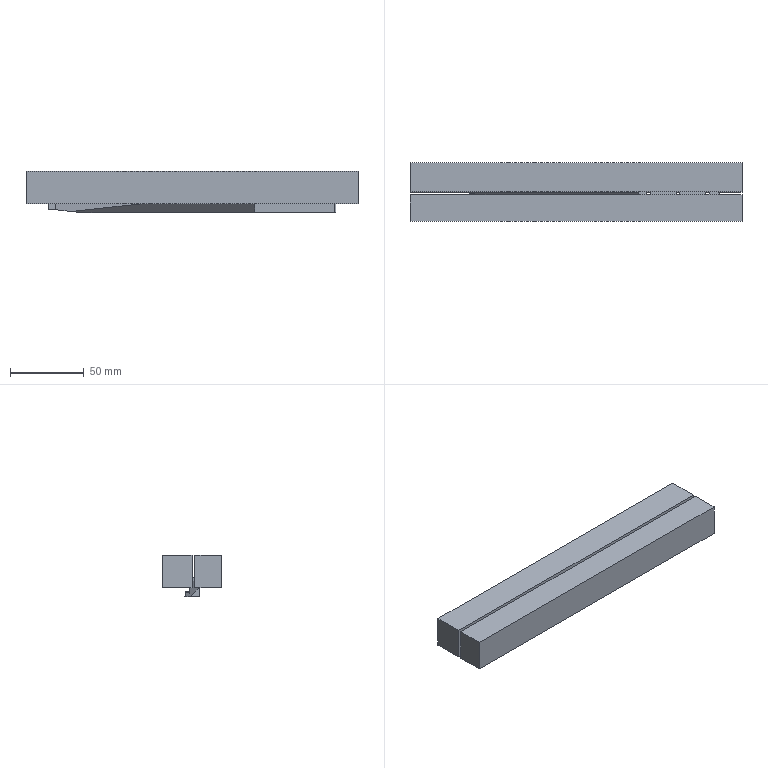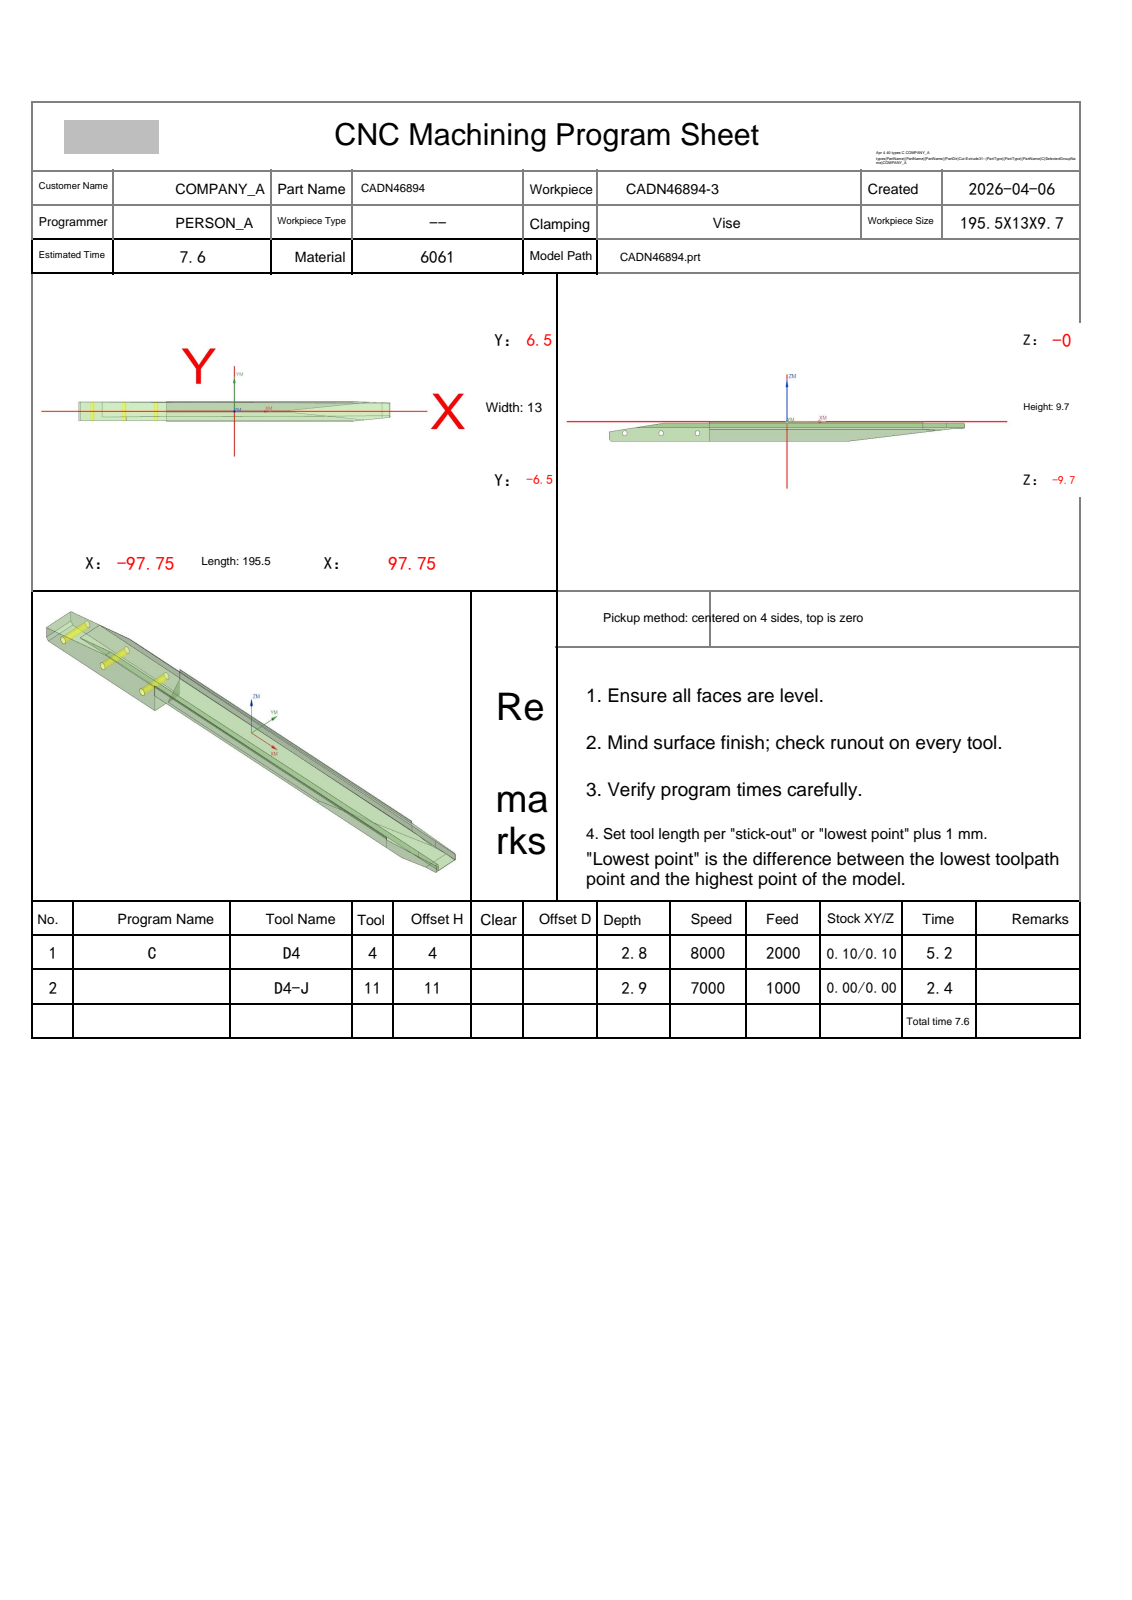NC program | NX | posted by the shop | part box 225.5 x 39.7 x 28 mm
Lines 11943 to 12871 of 20119:
N3 T19 M06
(D1.5-J  D=1.5 R=0. H=19 ce=0.00 di=0.00)
G00 G90 G54 X-194.982 Y-9.122 M03 S8000
G43 H19 Z44.
M08
Z-5.95
G01 X-194.984 Y-9.121 Z-5.973 F800.
X-194.989 Y-9.118 Z-5.993
X-194.996 Y-9.115 Z-6.012
X-195.007 Y-9.11 Z-6.028
X-195.02 Y-9.105 Z-6.042
X-195.034 Y-9.101 Z-6.055
X-195.05 Y-9.097 Z-6.065
X-195.068 Y-9.093 Z-6.074
X-195.086 Y-9.092 Z-6.082
X-195.105 Z-6.088
X-195.124 Y-9.094 Z-6.092
X-195.143 Y-9.099 Z-6.096
X-195.162 Y-9.108 Z-6.098
X-195.179 Y-9.119 Z-6.1
X-195.196 Y-9.135
G02 X-195.625 Y-9.483 I-1.304 J1.167
G03 X-195.75 Y-9.7 I.125 J-.217
X-195.5 Y-9.95 I.25 J0.0
G01 X-195.35 Y-9.9
G02 X-194.869 Y-9.583 I2.85 J-3.8
G01 X-194.848 Y-9.565 Z-6.101
X-194.834 Y-9.541 Z-6.102
X-194.824 Y-9.511 Z-6.105
X-194.82 Y-9.477 Z-6.108
Y-9.442 Z-6.112
X-194.823 Y-9.406 Z-6.117
X-194.828 Y-9.371 Z-6.122
X-194.836 Y-9.338 Z-6.127
X-194.851 Y-9.294 Z-6.136
X-194.871 Y-9.258 Z-6.145
X-194.895 Y-9.227 Z-6.155
X-194.927 Y-9.2 Z-6.164
X-194.966 Y-9.174 Z-6.173
X-194.994 Y-9.157 Z-6.178
X-195.025 Y-9.141 Z-6.183
X-195.057 Y-9.127 Z-6.188
X-195.089 Y-9.117 Z-6.192
X-195.12 Y-9.111 Z-6.195
X-195.149 Z-6.198
X-195.175 Y-9.119 Z-6.199
X-195.196 Y-9.135 Z-6.2
G02 X-195.625 Y-9.483 I-1.304 J1.167
G03 X-195.75 Y-9.7 I.125 J-.217
X-195.5 Y-9.95 I.25 J0.0
G01 X-195.35 Y-9.9
G02 X-194.869 Y-9.583 I2.85 J-3.8
G01 X-194.848 Y-9.565 Z-6.201
X-194.834 Y-9.541 Z-6.202
X-194.824 Y-9.511 Z-6.205
X-194.82 Y-9.477 Z-6.208
Y-9.442 Z-6.212
X-194.823 Y-9.406 Z-6.217
X-194.828 Y-9.371 Z-6.222
X-194.836 Y-9.338 Z-6.227
X-194.851 Y-9.294 Z-6.236
X-194.871 Y-9.258 Z-6.245
X-194.895 Y-9.227 Z-6.255
X-194.927 Y-9.2 Z-6.264
X-194.966 Y-9.174 Z-6.273
X-194.994 Y-9.157 Z-6.278
X-195.025 Y-9.141 Z-6.283
X-195.057 Y-9.127 Z-6.288
X-195.089 Y-9.117 Z-6.292
X-195.12 Y-9.111 Z-6.295
X-195.149 Z-6.298
X-195.175 Y-9.119 Z-6.299
X-195.196 Y-9.135 Z-6.3
G02 X-195.625 Y-9.483 I-1.304 J1.167
G03 X-195.75 Y-9.7 I.125 J-.217
X-195.5 Y-9.95 I.25 J0.0
G01 X-195.35 Y-9.9
G02 X-194.869 Y-9.583 I2.85 J-3.8
G01 X-194.848 Y-9.565 Z-6.301
X-194.834 Y-9.541 Z-6.302
X-194.824 Y-9.511 Z-6.305
X-194.82 Y-9.477 Z-6.308
Y-9.442 Z-6.312
X-194.823 Y-9.406 Z-6.317
X-194.828 Y-9.371 Z-6.322
X-194.836 Y-9.338 Z-6.327
X-194.851 Y-9.294 Z-6.336
X-194.871 Y-9.258 Z-6.345
X-194.895 Y-9.227 Z-6.355
X-194.927 Y-9.2 Z-6.364
X-194.966 Y-9.174 Z-6.373
X-194.994 Y-9.157 Z-6.378
X-195.025 Y-9.141 Z-6.383
X-195.057 Y-9.127 Z-6.388
X-195.089 Y-9.117 Z-6.392
X-195.12 Y-9.111 Z-6.395
X-195.149 Z-6.398
X-195.175 Y-9.119 Z-6.399
X-195.196 Y-9.135 Z-6.4
G02 X-195.625 Y-9.483 I-1.304 J1.167
G03 X-195.75 Y-9.7 I.125 J-.217
X-195.5 Y-9.95 I.25 J0.0
G01 X-195.35 Y-9.9
G02 X-194.869 Y-9.583 I2.85 J-3.8
G01 X-194.848 Y-9.565 Z-6.401
X-194.834 Y-9.541 Z-6.402
X-194.824 Y-9.511 Z-6.405
X-194.82 Y-9.477 Z-6.408
Y-9.442 Z-6.412
X-194.823 Y-9.406 Z-6.417
X-194.828 Y-9.371 Z-6.422
X-194.836 Y-9.338 Z-6.427
X-194.851 Y-9.294 Z-6.436
X-194.871 Y-9.258 Z-6.445
X-194.895 Y-9.227 Z-6.455
X-194.927 Y-9.2 Z-6.464
X-194.966 Y-9.174 Z-6.473
X-194.994 Y-9.157 Z-6.478
X-195.025 Y-9.141 Z-6.483
X-195.057 Y-9.127 Z-6.488
X-195.089 Y-9.117 Z-6.492
X-195.12 Y-9.111 Z-6.495
X-195.149 Z-6.498
X-195.175 Y-9.119 Z-6.499
X-195.196 Y-9.135 Z-6.5
G02 X-195.625 Y-9.483 I-1.304 J1.167
G03 X-195.75 Y-9.7 I.125 J-.217
X-195.5 Y-9.95 I.25 J0.0
G01 X-195.35 Y-9.9
G02 X-194.869 Y-9.583 I2.85 J-3.8
G01 X-194.848 Y-9.565 Z-6.501
X-194.834 Y-9.541 Z-6.502
X-194.824 Y-9.511 Z-6.505
X-194.82 Y-9.477 Z-6.508
Y-9.442 Z-6.512
X-194.823 Y-9.406 Z-6.517
X-194.828 Y-9.371 Z-6.522
X-194.836 Y-9.338 Z-6.527
X-194.851 Y-9.294 Z-6.536
X-194.871 Y-9.258 Z-6.545
X-194.895 Y-9.227 Z-6.555
X-194.927 Y-9.2 Z-6.564
X-194.966 Y-9.174 Z-6.573
X-194.994 Y-9.157 Z-6.578
X-195.025 Y-9.141 Z-6.583
X-195.057 Y-9.127 Z-6.588
X-195.089 Y-9.117 Z-6.592
X-195.12 Y-9.111 Z-6.595
X-195.149 Z-6.598
X-195.175 Y-9.119 Z-6.599
X-195.196 Y-9.135 Z-6.6
G02 X-195.625 Y-9.483 I-1.304 J1.167
G03 X-195.75 Y-9.7 I.125 J-.217
X-195.5 Y-9.95 I.25 J0.0
G01 X-195.35 Y-9.9
G02 X-194.869 Y-9.583 I2.85 J-3.8
G01 X-194.848 Y-9.565 Z-6.601
X-194.834 Y-9.541 Z-6.602
X-194.824 Y-9.511 Z-6.605
X-194.82 Y-9.477 Z-6.608
Y-9.442 Z-6.612
X-194.823 Y-9.406 Z-6.617
X-194.828 Y-9.371 Z-6.622
X-194.836 Y-9.338 Z-6.627
X-194.851 Y-9.294 Z-6.636
X-194.871 Y-9.258 Z-6.645
X-194.895 Y-9.227 Z-6.655
X-194.927 Y-9.2 Z-6.664
X-194.966 Y-9.174 Z-6.673
X-194.994 Y-9.157 Z-6.678
X-195.025 Y-9.141 Z-6.683
X-195.057 Y-9.127 Z-6.688
X-195.089 Y-9.117 Z-6.692
X-195.12 Y-9.111 Z-6.695
X-195.149 Z-6.698
X-195.175 Y-9.119 Z-6.699
X-195.196 Y-9.135 Z-6.7
G02 X-195.625 Y-9.483 I-1.304 J1.167
G03 X-195.75 Y-9.7 I.125 J-.217
X-195.5 Y-9.95 I.25 J0.0
G01 X-195.35 Y-9.9
G02 X-194.869 Y-9.583 I2.85 J-3.8
G01 X-194.848 Y-9.565 Z-6.701
X-194.834 Y-9.541 Z-6.702
X-194.824 Y-9.511 Z-6.705
X-194.82 Y-9.477 Z-6.708
Y-9.442 Z-6.712
X-194.823 Y-9.406 Z-6.717
X-194.828 Y-9.371 Z-6.722
X-194.836 Y-9.338 Z-6.727
X-194.851 Y-9.294 Z-6.736
X-194.871 Y-9.258 Z-6.745
X-194.895 Y-9.227 Z-6.755
X-194.927 Y-9.2 Z-6.764
X-194.966 Y-9.174 Z-6.773
X-194.994 Y-9.157 Z-6.778
X-195.025 Y-9.141 Z-6.783
X-195.057 Y-9.127 Z-6.788
X-195.089 Y-9.117 Z-6.792
X-195.12 Y-9.111 Z-6.795
X-195.149 Z-6.798
X-195.175 Y-9.119 Z-6.799
X-195.196 Y-9.135 Z-6.8
G02 X-195.625 Y-9.483 I-1.304 J1.167
G03 X-195.75 Y-9.7 I.125 J-.217
X-195.5 Y-9.95 I.25 J0.0
G01 X-195.35 Y-9.9
G02 X-194.869 Y-9.583 I2.85 J-3.8
G01 X-194.848 Y-9.565 Z-6.801
X-194.834 Y-9.541 Z-6.802
X-194.824 Y-9.511 Z-6.805
X-194.82 Y-9.477 Z-6.808
Y-9.442 Z-6.812
X-194.823 Y-9.406 Z-6.817
X-194.828 Y-9.371 Z-6.822
X-194.836 Y-9.338 Z-6.827
X-194.851 Y-9.294 Z-6.836
X-194.871 Y-9.258 Z-6.845
X-194.895 Y-9.227 Z-6.855
X-194.927 Y-9.2 Z-6.864
X-194.966 Y-9.174 Z-6.873
X-194.994 Y-9.157 Z-6.878
X-195.025 Y-9.141 Z-6.883
X-195.057 Y-9.127 Z-6.888
X-195.089 Y-9.117 Z-6.892
X-195.12 Y-9.111 Z-6.895
X-195.149 Z-6.898
X-195.175 Y-9.119 Z-6.899
X-195.196 Y-9.135 Z-6.9
G02 X-195.625 Y-9.483 I-1.304 J1.167
G03 X-195.75 Y-9.7 I.125 J-.217
X-195.5 Y-9.95 I.25 J0.0
G01 X-195.35 Y-9.9
G02 X-194.869 Y-9.583 I2.85 J-3.8
G01 X-194.848 Y-9.565 Z-6.901
X-194.834 Y-9.541 Z-6.902
X-194.824 Y-9.511 Z-6.905
X-194.82 Y-9.477 Z-6.908
Y-9.442 Z-6.912
X-194.823 Y-9.406 Z-6.917
X-194.828 Y-9.371 Z-6.922
X-194.836 Y-9.338 Z-6.927
X-194.851 Y-9.294 Z-6.936
X-194.871 Y-9.258 Z-6.945
X-194.895 Y-9.227 Z-6.955
X-194.927 Y-9.2 Z-6.964
X-194.966 Y-9.174 Z-6.973
X-194.994 Y-9.157 Z-6.978
X-195.025 Y-9.141 Z-6.983
X-195.057 Y-9.127 Z-6.988
X-195.089 Y-9.117 Z-6.992
X-195.12 Y-9.111 Z-6.995
X-195.149 Z-6.998
X-195.175 Y-9.119 Z-6.999
X-195.196 Y-9.135 Z-7.
G02 X-195.625 Y-9.483 I-1.304 J1.167
G03 X-195.75 Y-9.7 I.125 J-.217
X-195.5 Y-9.95 I.25 J0.0
G01 X-195.35 Y-9.9
G02 X-194.869 Y-9.583 I2.85 J-3.8
G01 X-194.848 Y-9.565 Z-7.001
X-194.834 Y-9.541 Z-7.002
X-194.824 Y-9.511 Z-7.005
X-194.82 Y-9.477 Z-7.008
Y-9.442 Z-7.012
X-194.823 Y-9.406 Z-7.017
X-194.828 Y-9.371 Z-7.022
X-194.836 Y-9.338 Z-7.027
X-194.851 Y-9.294 Z-7.036
X-194.871 Y-9.258 Z-7.045
X-194.895 Y-9.227 Z-7.055
X-194.927 Y-9.2 Z-7.064
X-194.966 Y-9.174 Z-7.073
X-194.994 Y-9.157 Z-7.078
X-195.025 Y-9.141 Z-7.083
X-195.057 Y-9.127 Z-7.088
X-195.089 Y-9.117 Z-7.092
X-195.12 Y-9.111 Z-7.095
X-195.149 Z-7.098
X-195.175 Y-9.119 Z-7.099
X-195.196 Y-9.135 Z-7.1
G02 X-195.625 Y-9.483 I-1.304 J1.167
G03 X-195.75 Y-9.7 I.125 J-.217
X-195.5 Y-9.95 I.25 J0.0
G01 X-195.35 Y-9.9
G02 X-194.869 Y-9.583 I2.85 J-3.8
G01 X-194.848 Y-9.565 Z-7.101
X-194.834 Y-9.541 Z-7.102
X-194.824 Y-9.511 Z-7.105
X-194.82 Y-9.477 Z-7.108
Y-9.442 Z-7.112
X-194.823 Y-9.406 Z-7.117
X-194.828 Y-9.371 Z-7.122
X-194.836 Y-9.338 Z-7.127
X-194.851 Y-9.294 Z-7.136
X-194.871 Y-9.258 Z-7.145
X-194.895 Y-9.227 Z-7.155
X-194.927 Y-9.2 Z-7.164
X-194.966 Y-9.174 Z-7.173
X-194.994 Y-9.157 Z-7.178
X-195.025 Y-9.141 Z-7.183
X-195.057 Y-9.127 Z-7.188
X-195.089 Y-9.117 Z-7.192
X-195.12 Y-9.111 Z-7.195
X-195.149 Z-7.198
X-195.175 Y-9.119 Z-7.199
X-195.196 Y-9.135 Z-7.2
G02 X-195.625 Y-9.483 I-1.304 J1.167
G03 X-195.75 Y-9.7 I.125 J-.217
X-195.5 Y-9.95 I.25 J0.0
G01 X-195.35 Y-9.9
G02 X-194.869 Y-9.583 I2.85 J-3.8
G01 X-194.848 Y-9.565 Z-7.201
X-194.834 Y-9.541 Z-7.202
X-194.824 Y-9.511 Z-7.205
X-194.82 Y-9.477 Z-7.208
Y-9.442 Z-7.212
X-194.823 Y-9.406 Z-7.217
X-194.828 Y-9.371 Z-7.222
X-194.836 Y-9.338 Z-7.227
X-194.851 Y-9.294 Z-7.236
X-194.871 Y-9.258 Z-7.245
X-194.895 Y-9.227 Z-7.255
X-194.927 Y-9.2 Z-7.264
X-194.966 Y-9.174 Z-7.273
X-194.994 Y-9.157 Z-7.278
X-195.025 Y-9.141 Z-7.283
X-195.057 Y-9.127 Z-7.288
X-195.089 Y-9.117 Z-7.292
X-195.12 Y-9.111 Z-7.295
X-195.149 Z-7.298
X-195.175 Y-9.119 Z-7.299
X-195.196 Y-9.135 Z-7.3
G02 X-195.625 Y-9.483 I-1.304 J1.167
G03 X-195.75 Y-9.7 I.125 J-.217
X-195.5 Y-9.95 I.25 J0.0
G01 X-195.35 Y-9.9
G02 X-194.869 Y-9.583 I2.85 J-3.8
G01 X-194.848 Y-9.565 Z-7.301
X-194.834 Y-9.541 Z-7.302
X-194.824 Y-9.511 Z-7.305
X-194.82 Y-9.477 Z-7.308
Y-9.442 Z-7.312
X-194.823 Y-9.406 Z-7.317
X-194.828 Y-9.371 Z-7.322
X-194.836 Y-9.338 Z-7.327
X-194.851 Y-9.294 Z-7.336
X-194.871 Y-9.258 Z-7.345
X-194.895 Y-9.227 Z-7.355
X-194.927 Y-9.2 Z-7.364
X-194.966 Y-9.174 Z-7.373
X-194.994 Y-9.157 Z-7.378
X-195.025 Y-9.141 Z-7.383
X-195.057 Y-9.127 Z-7.388
X-195.089 Y-9.117 Z-7.392
X-195.12 Y-9.111 Z-7.395
X-195.149 Z-7.398
X-195.175 Y-9.119 Z-7.399
X-195.196 Y-9.135 Z-7.4
G02 X-195.625 Y-9.483 I-1.304 J1.167
G03 X-195.75 Y-9.7 I.125 J-.217
X-195.5 Y-9.95 I.25 J0.0
G01 X-195.35 Y-9.9
G02 X-194.869 Y-9.583 I2.85 J-3.8
G01 X-194.848 Y-9.565 Z-7.401
X-194.834 Y-9.541 Z-7.402
X-194.824 Y-9.511 Z-7.405
X-194.82 Y-9.477 Z-7.408
Y-9.442 Z-7.412
X-194.823 Y-9.406 Z-7.417
X-194.828 Y-9.371 Z-7.422
X-194.836 Y-9.338 Z-7.427
X-194.851 Y-9.294 Z-7.436
X-194.871 Y-9.258 Z-7.445
X-194.895 Y-9.227 Z-7.455
X-194.927 Y-9.2 Z-7.464
X-194.966 Y-9.174 Z-7.473
X-194.994 Y-9.157 Z-7.478
X-195.025 Y-9.141 Z-7.483
X-195.057 Y-9.127 Z-7.488
X-195.089 Y-9.117 Z-7.492
X-195.12 Y-9.111 Z-7.495
X-195.149 Z-7.498
X-195.175 Y-9.119 Z-7.499
X-195.196 Y-9.135 Z-7.5
G02 X-195.625 Y-9.483 I-1.304 J1.167
G03 X-195.75 Y-9.7 I.125 J-.217
X-195.5 Y-9.95 I.25 J0.0
G01 X-195.35 Y-9.9
G02 X-194.869 Y-9.583 I2.85 J-3.8
G01 X-194.848 Y-9.565 Z-7.501
X-194.834 Y-9.541 Z-7.502
X-194.824 Y-9.511 Z-7.505
X-194.82 Y-9.477 Z-7.508
Y-9.442 Z-7.512
X-194.823 Y-9.406 Z-7.517
X-194.828 Y-9.371 Z-7.522
X-194.836 Y-9.338 Z-7.527
X-194.851 Y-9.294 Z-7.536
X-194.871 Y-9.258 Z-7.545
X-194.895 Y-9.227 Z-7.555
X-194.927 Y-9.2 Z-7.564
X-194.966 Y-9.174 Z-7.573
X-194.994 Y-9.157 Z-7.578
X-195.025 Y-9.141 Z-7.583
X-195.057 Y-9.127 Z-7.588
X-195.089 Y-9.117 Z-7.592
X-195.12 Y-9.111 Z-7.595
X-195.149 Z-7.598
X-195.175 Y-9.119 Z-7.599
X-195.196 Y-9.135 Z-7.6
G02 X-195.625 Y-9.483 I-1.304 J1.167
G03 X-195.75 Y-9.7 I.125 J-.217
X-195.5 Y-9.95 I.25 J0.0
G01 X-195.35 Y-9.9
G02 X-194.869 Y-9.583 I2.85 J-3.8
G01 X-194.848 Y-9.565 Z-7.601
X-194.834 Y-9.541 Z-7.602
X-194.824 Y-9.511 Z-7.605
X-194.82 Y-9.477 Z-7.608
Y-9.442 Z-7.612
X-194.823 Y-9.406 Z-7.617
X-194.828 Y-9.371 Z-7.622
X-194.836 Y-9.338 Z-7.627
X-194.851 Y-9.294 Z-7.636
X-194.871 Y-9.258 Z-7.645
X-194.895 Y-9.227 Z-7.655
X-194.927 Y-9.2 Z-7.664
X-194.966 Y-9.174 Z-7.673
X-194.994 Y-9.157 Z-7.678
X-195.025 Y-9.141 Z-7.683
X-195.057 Y-9.127 Z-7.688
X-195.089 Y-9.117 Z-7.692
X-195.12 Y-9.111 Z-7.695
X-195.149 Z-7.698
X-195.175 Y-9.119 Z-7.699
X-195.196 Y-9.135 Z-7.7
G02 X-195.625 Y-9.483 I-1.304 J1.167
G03 X-195.75 Y-9.7 I.125 J-.217
X-195.5 Y-9.95 I.25 J0.0
G01 X-195.35 Y-9.9
G02 X-194.869 Y-9.583 I2.85 J-3.8
G01 X-194.848 Y-9.565 Z-7.701
X-194.834 Y-9.541 Z-7.702
X-194.824 Y-9.511 Z-7.705
X-194.82 Y-9.477 Z-7.708
Y-9.442 Z-7.712
X-194.823 Y-9.406 Z-7.717
X-194.828 Y-9.371 Z-7.722
X-194.836 Y-9.338 Z-7.727
X-194.851 Y-9.294 Z-7.736
X-194.871 Y-9.258 Z-7.745
X-194.895 Y-9.227 Z-7.755
X-194.927 Y-9.2 Z-7.764
X-194.966 Y-9.174 Z-7.773
X-194.994 Y-9.157 Z-7.778
X-195.025 Y-9.141 Z-7.783
X-195.057 Y-9.127 Z-7.788
X-195.089 Y-9.117 Z-7.792
X-195.12 Y-9.111 Z-7.795
X-195.149 Z-7.798
X-195.175 Y-9.119 Z-7.799
X-195.196 Y-9.135 Z-7.8
G02 X-195.625 Y-9.483 I-1.304 J1.167
G03 X-195.75 Y-9.7 I.125 J-.217
X-195.5 Y-9.95 I.25 J0.0
G01 X-195.35 Y-9.9
G02 X-194.869 Y-9.583 I2.85 J-3.8
G01 X-194.848 Y-9.565 Z-7.801
X-194.834 Y-9.541 Z-7.802
X-194.824 Y-9.511 Z-7.805
X-194.82 Y-9.477 Z-7.808
Y-9.442 Z-7.812
X-194.823 Y-9.406 Z-7.817
X-194.828 Y-9.371 Z-7.822
X-194.836 Y-9.338 Z-7.827
X-194.851 Y-9.294 Z-7.836
X-194.871 Y-9.258 Z-7.845
X-194.895 Y-9.227 Z-7.855
X-194.927 Y-9.2 Z-7.864
X-194.966 Y-9.174 Z-7.873
X-194.994 Y-9.157 Z-7.878
X-195.025 Y-9.141 Z-7.883
X-195.057 Y-9.127 Z-7.888
X-195.089 Y-9.117 Z-7.892
X-195.12 Y-9.111 Z-7.895
X-195.149 Z-7.898
X-195.175 Y-9.119 Z-7.899
X-195.196 Y-9.135 Z-7.9
G02 X-195.625 Y-9.483 I-1.304 J1.167
G03 X-195.75 Y-9.7 I.125 J-.217
X-195.5 Y-9.95 I.25 J0.0
G01 X-195.35 Y-9.9
G02 X-194.869 Y-9.583 I2.85 J-3.8
G01 X-194.848 Y-9.565 Z-7.901
X-194.834 Y-9.541 Z-7.902
X-194.824 Y-9.511 Z-7.905
X-194.82 Y-9.477 Z-7.908
Y-9.442 Z-7.912
X-194.823 Y-9.406 Z-7.917
X-194.828 Y-9.371 Z-7.922
X-194.836 Y-9.338 Z-7.927
X-194.851 Y-9.294 Z-7.936
X-194.871 Y-9.258 Z-7.945
X-194.895 Y-9.227 Z-7.955
X-194.927 Y-9.2 Z-7.964
X-194.966 Y-9.174 Z-7.973
X-194.994 Y-9.157 Z-7.978
X-195.025 Y-9.141 Z-7.983
X-195.057 Y-9.127 Z-7.988
X-195.089 Y-9.117 Z-7.992
X-195.12 Y-9.111 Z-7.995
X-195.149 Z-7.998
X-195.175 Y-9.119 Z-7.999
X-195.196 Y-9.135 Z-8.
G02 X-195.625 Y-9.483 I-1.304 J1.167
G03 X-195.75 Y-9.7 I.125 J-.217
X-195.5 Y-9.95 I.25 J0.0
G01 X-195.35 Y-9.9
G02 X-194.869 Y-9.583 I2.85 J-3.8
G01 X-194.848 Y-9.565 Z-8.001
X-194.834 Y-9.541 Z-8.002
X-194.824 Y-9.511 Z-8.005
X-194.82 Y-9.477 Z-8.008
Y-9.442 Z-8.012
X-194.823 Y-9.406 Z-8.017
X-194.828 Y-9.371 Z-8.022
X-194.836 Y-9.338 Z-8.027
X-194.851 Y-9.294 Z-8.036
X-194.871 Y-9.258 Z-8.045
X-194.895 Y-9.227 Z-8.055
X-194.927 Y-9.2 Z-8.064
X-194.966 Y-9.174 Z-8.073
X-194.994 Y-9.157 Z-8.078
X-195.025 Y-9.141 Z-8.083
X-195.057 Y-9.127 Z-8.088
X-195.089 Y-9.117 Z-8.092
X-195.12 Y-9.111 Z-8.095
X-195.149 Z-8.098
X-195.175 Y-9.119 Z-8.099
X-195.196 Y-9.135 Z-8.1
G02 X-195.625 Y-9.483 I-1.304 J1.167
G03 X-195.75 Y-9.7 I.125 J-.217
X-195.5 Y-9.95 I.25 J0.0
G01 X-195.35 Y-9.9
G02 X-194.869 Y-9.583 I2.85 J-3.8
G01 X-194.848 Y-9.565 Z-8.101
X-194.834 Y-9.541 Z-8.102
X-194.824 Y-9.511 Z-8.105
X-194.82 Y-9.477 Z-8.108
Y-9.442 Z-8.112
X-194.823 Y-9.406 Z-8.117
X-194.828 Y-9.371 Z-8.122
X-194.836 Y-9.338 Z-8.127
X-194.851 Y-9.294 Z-8.136
X-194.871 Y-9.258 Z-8.145
X-194.895 Y-9.227 Z-8.155
X-194.927 Y-9.2 Z-8.164
X-194.966 Y-9.174 Z-8.173
X-194.994 Y-9.157 Z-8.178
X-195.025 Y-9.141 Z-8.183
X-195.057 Y-9.127 Z-8.188
X-195.089 Y-9.117 Z-8.192
X-195.12 Y-9.111 Z-8.195
X-195.149 Z-8.198
X-195.175 Y-9.119 Z-8.199
X-195.196 Y-9.135 Z-8.2
G02 X-195.625 Y-9.483 I-1.304 J1.167
G03 X-195.75 Y-9.7 I.125 J-.217
X-195.5 Y-9.95 I.25 J0.0
G01 X-195.35 Y-9.9
G02 X-194.869 Y-9.583 I2.85 J-3.8
G01 X-194.848 Y-9.565 Z-8.201
X-194.834 Y-9.541 Z-8.202
X-194.824 Y-9.511 Z-8.205
X-194.82 Y-9.477 Z-8.208
Y-9.442 Z-8.212
X-194.823 Y-9.406 Z-8.217
X-194.828 Y-9.371 Z-8.222
X-194.836 Y-9.338 Z-8.227
X-194.851 Y-9.294 Z-8.236
X-194.871 Y-9.258 Z-8.245
X-194.895 Y-9.227 Z-8.255
X-194.927 Y-9.2 Z-8.264
X-194.966 Y-9.174 Z-8.273
X-194.994 Y-9.157 Z-8.278
X-195.025 Y-9.141 Z-8.283
X-195.057 Y-9.127 Z-8.288
X-195.089 Y-9.117 Z-8.292
X-195.12 Y-9.111 Z-8.295
X-195.149 Z-8.298
X-195.175 Y-9.119 Z-8.299
X-195.196 Y-9.135 Z-8.3
G02 X-195.625 Y-9.483 I-1.304 J1.167
G03 X-195.75 Y-9.7 I.125 J-.217
X-195.5 Y-9.95 I.25 J0.0
G01 X-195.35 Y-9.9
G02 X-194.869 Y-9.583 I2.85 J-3.8
G01 X-194.848 Y-9.565 Z-8.301
X-194.834 Y-9.541 Z-8.302
X-194.824 Y-9.511 Z-8.305
X-194.82 Y-9.477 Z-8.308
Y-9.442 Z-8.312
X-194.823 Y-9.406 Z-8.317
X-194.828 Y-9.371 Z-8.322
X-194.836 Y-9.338 Z-8.327
X-194.851 Y-9.294 Z-8.336
X-194.871 Y-9.258 Z-8.345
X-194.895 Y-9.227 Z-8.355
X-194.927 Y-9.2 Z-8.364
X-194.966 Y-9.174 Z-8.373
X-194.994 Y-9.157 Z-8.378
X-195.025 Y-9.141 Z-8.383
X-195.057 Y-9.127 Z-8.388
X-195.089 Y-9.117 Z-8.392
X-195.12 Y-9.111 Z-8.395
X-195.149 Z-8.398
X-195.175 Y-9.119 Z-8.399
X-195.196 Y-9.135 Z-8.4
G02 X-195.625 Y-9.483 I-1.304 J1.167
G03 X-195.75 Y-9.7 I.125 J-.217
X-195.5 Y-9.95 I.25 J0.0
G01 X-195.35 Y-9.9
G02 X-194.869 Y-9.583 I2.85 J-3.8
G01 X-194.848 Y-9.565 Z-8.401
X-194.834 Y-9.541 Z-8.402
X-194.824 Y-9.511 Z-8.405
X-194.82 Y-9.477 Z-8.408
Y-9.442 Z-8.412
X-194.823 Y-9.406 Z-8.417
X-194.828 Y-9.371 Z-8.422
X-194.836 Y-9.338 Z-8.427
X-194.851 Y-9.294 Z-8.436
X-194.871 Y-9.258 Z-8.445
X-194.895 Y-9.227 Z-8.455
X-194.927 Y-9.2 Z-8.464
X-194.966 Y-9.174 Z-8.473
X-194.994 Y-9.157 Z-8.478
X-195.025 Y-9.141 Z-8.483
X-195.057 Y-9.127 Z-8.488
X-195.089 Y-9.117 Z-8.492
X-195.12 Y-9.111 Z-8.495
X-195.149 Z-8.498
X-195.175 Y-9.119 Z-8.499
X-195.196 Y-9.135 Z-8.5
G02 X-195.625 Y-9.483 I-1.304 J1.167
G03 X-195.75 Y-9.7 I.125 J-.217
X-195.5 Y-9.95 I.25 J0.0
G01 X-195.35 Y-9.9
G02 X-194.869 Y-9.583 I2.85 J-3.8
G01 X-194.848 Y-9.565 Z-8.501
X-194.834 Y-9.541 Z-8.502
X-194.824 Y-9.511 Z-8.505
X-194.82 Y-9.477 Z-8.508
Y-9.442 Z-8.512
X-194.823 Y-9.406 Z-8.517
X-194.828 Y-9.371 Z-8.522
X-194.836 Y-9.338 Z-8.527
X-194.851 Y-9.294 Z-8.536
X-194.871 Y-9.258 Z-8.545
X-194.895 Y-9.227 Z-8.555
X-194.927 Y-9.2 Z-8.564
X-194.966 Y-9.174 Z-8.573
X-194.994 Y-9.157 Z-8.578
X-195.025 Y-9.141 Z-8.583
X-195.057 Y-9.127 Z-8.588
X-195.089 Y-9.117 Z-8.592
X-195.12 Y-9.111 Z-8.595
X-195.149 Z-8.598
X-195.175 Y-9.119 Z-8.599
X-195.196 Y-9.135 Z-8.6
G02 X-195.625 Y-9.483 I-1.304 J1.167
G03 X-195.75 Y-9.7 I.125 J-.217
X-195.5 Y-9.95 I.25 J0.0
G01 X-195.35 Y-9.9
G02 X-194.869 Y-9.583 I2.85 J-3.8
G01 X-194.848 Y-9.565 Z-8.601
X-194.834 Y-9.541 Z-8.602
X-194.824 Y-9.511 Z-8.605
X-194.82 Y-9.477 Z-8.608
Y-9.442 Z-8.612
X-194.823 Y-9.406 Z-8.617
X-194.828 Y-9.371 Z-8.622
X-194.836 Y-9.338 Z-8.627
X-194.851 Y-9.294 Z-8.636
X-194.871 Y-9.258 Z-8.645
X-194.895 Y-9.227 Z-8.655
X-194.927 Y-9.2 Z-8.664
X-194.966 Y-9.174 Z-8.673
X-194.994 Y-9.157 Z-8.678
X-195.025 Y-9.141 Z-8.683
X-195.057 Y-9.127 Z-8.688
X-195.089 Y-9.117 Z-8.692
X-195.12 Y-9.111 Z-8.695
X-195.149 Z-8.698
X-195.175 Y-9.119 Z-8.699
X-195.196 Y-9.135 Z-8.7
G02 X-195.625 Y-9.483 I-1.304 J1.167
G03 X-195.75 Y-9.7 I.125 J-.217
X-195.5 Y-9.95 I.25 J0.0
G01 X-195.35 Y-9.9
G02 X-194.869 Y-9.583 I2.85 J-3.8
G01 X-194.848 Y-9.565 Z-8.701
X-194.834 Y-9.541 Z-8.702
X-194.824 Y-9.511 Z-8.705
X-194.82 Y-9.477 Z-8.708
Y-9.442 Z-8.712
X-194.823 Y-9.406 Z-8.717
X-194.828 Y-9.371 Z-8.722
X-194.836 Y-9.338 Z-8.727
X-194.851 Y-9.294 Z-8.736
X-194.871 Y-9.258 Z-8.745
X-194.895 Y-9.227 Z-8.755
X-194.927 Y-9.2 Z-8.764
X-194.966 Y-9.174 Z-8.773
X-194.994 Y-9.157 Z-8.778
X-195.025 Y-9.141 Z-8.783
X-195.057 Y-9.127 Z-8.788
X-195.089 Y-9.117 Z-8.792
X-195.12 Y-9.111 Z-8.795
X-195.149 Z-8.798
X-195.175 Y-9.119 Z-8.799
X-195.196 Y-9.135 Z-8.8
G02 X-195.625 Y-9.483 I-1.304 J1.167
G03 X-195.75 Y-9.7 I.125 J-.217
X-195.5 Y-9.95 I.25 J0.0
G01 X-195.35 Y-9.9
G02 X-194.869 Y-9.583 I2.85 J-3.8
G01 X-194.848 Y-9.565 Z-8.801
X-194.834 Y-9.541 Z-8.802
X-194.824 Y-9.511 Z-8.805
X-194.82 Y-9.477 Z-8.808
Y-9.442 Z-8.812
X-194.823 Y-9.406 Z-8.817
X-194.828 Y-9.371 Z-8.822
X-194.836 Y-9.338 Z-8.827
X-194.851 Y-9.294 Z-8.836
X-194.871 Y-9.258 Z-8.845
X-194.895 Y-9.227 Z-8.855
X-194.927 Y-9.2 Z-8.864
X-194.966 Y-9.174 Z-8.873
X-194.994 Y-9.157 Z-8.878
X-195.025 Y-9.141 Z-8.883
X-195.057 Y-9.127 Z-8.888
X-195.089 Y-9.117 Z-8.892
X-195.12 Y-9.111 Z-8.895
X-195.149 Z-8.898
X-195.175 Y-9.119 Z-8.899
X-195.196 Y-9.135 Z-8.9
G02 X-195.625 Y-9.483 I-1.304 J1.167
G03 X-195.75 Y-9.7 I.125 J-.217
X-195.5 Y-9.95 I.25 J0.0
G01 X-195.35 Y-9.9
G02 X-194.869 Y-9.583 I2.85 J-3.8
G01 X-194.848 Y-9.565 Z-8.901
X-194.834 Y-9.541 Z-8.902
X-194.824 Y-9.511 Z-8.905
X-194.82 Y-9.477 Z-8.908
Y-9.442 Z-8.912
X-194.823 Y-9.406 Z-8.917
X-194.828 Y-9.371 Z-8.922
X-194.836 Y-9.338 Z-8.927
X-194.851 Y-9.294 Z-8.936
X-194.871 Y-9.258 Z-8.945
X-194.895 Y-9.227 Z-8.955
X-194.927 Y-9.2 Z-8.964
X-194.966 Y-9.174 Z-8.973
X-194.994 Y-9.157 Z-8.978
X-195.025 Y-9.141 Z-8.983
X-195.057 Y-9.127 Z-8.988
X-195.089 Y-9.117 Z-8.992
X-195.12 Y-9.111 Z-8.995
X-195.149 Z-8.998
X-195.175 Y-9.119 Z-8.999
X-195.196 Y-9.135 Z-9.
G02 X-195.625 Y-9.483 I-1.304 J1.167
G03 X-195.75 Y-9.7 I.125 J-.217
X-195.5 Y-9.95 I.25 J0.0
G01 X-195.35 Y-9.9
G02 X-194.869 Y-9.583 I2.85 J-3.8
G01 X-194.848 Y-9.565 Z-9.001
X-194.834 Y-9.541 Z-9.002
X-194.824 Y-9.511 Z-9.005
X-194.82 Y-9.477 Z-9.008
Y-9.442 Z-9.012
X-194.823 Y-9.406 Z-9.017
X-194.828 Y-9.371 Z-9.022
X-194.836 Y-9.338 Z-9.027
X-194.851 Y-9.294 Z-9.036
X-194.871 Y-9.258 Z-9.045
X-194.895 Y-9.227 Z-9.055
X-194.927 Y-9.2 Z-9.064
X-194.966 Y-9.174 Z-9.073
X-194.994 Y-9.157 Z-9.078
X-195.025 Y-9.141 Z-9.083
X-195.057 Y-9.127 Z-9.088
X-195.089 Y-9.117 Z-9.092
X-195.12 Y-9.111 Z-9.095
X-195.149 Z-9.098
X-195.175 Y-9.119 Z-9.099
X-195.196 Y-9.135 Z-9.1
G02 X-195.625 Y-9.483 I-1.304 J1.167
G03 X-195.75 Y-9.7 I.125 J-.217
X-195.5 Y-9.95 I.25 J0.0
G01 X-195.35 Y-9.9
G02 X-194.869 Y-9.583 I2.85 J-3.8
G01 X-194.848 Y-9.565 Z-9.101
X-194.834 Y-9.541 Z-9.102
X-194.824 Y-9.511 Z-9.105
X-194.82 Y-9.477 Z-9.108
Y-9.442 Z-9.112
X-194.823 Y-9.406 Z-9.117
X-194.828 Y-9.371 Z-9.122
X-194.836 Y-9.338 Z-9.127
X-194.851 Y-9.294 Z-9.136
X-194.871 Y-9.258 Z-9.145
X-194.895 Y-9.227 Z-9.155
X-194.927 Y-9.2 Z-9.164
X-194.966 Y-9.174 Z-9.173
X-194.994 Y-9.157 Z-9.178
X-195.025 Y-9.141 Z-9.183
X-195.057 Y-9.127 Z-9.188
X-195.089 Y-9.117 Z-9.192
X-195.12 Y-9.111 Z-9.195
X-195.149 Z-9.198
X-195.175 Y-9.119 Z-9.199
X-195.196 Y-9.135 Z-9.2
G02 X-195.625 Y-9.483 I-1.304 J1.167
G03 X-195.75 Y-9.7 I.125 J-.217
X-195.5 Y-9.95 I.25 J0.0
G01 X-195.35 Y-9.9
G02 X-194.869 Y-9.583 I2.85 J-3.8
G01 X-194.848 Y-9.565 Z-9.201
X-194.834 Y-9.541 Z-9.202
X-194.824 Y-9.511 Z-9.205
X-194.82 Y-9.477 Z-9.208
Y-9.442 Z-9.212
X-194.823 Y-9.406 Z-9.217
X-194.828 Y-9.371 Z-9.222
X-194.836 Y-9.338 Z-9.227
X-194.851 Y-9.294 Z-9.236
X-194.871 Y-9.258 Z-9.245
X-194.895 Y-9.227 Z-9.255
X-194.927 Y-9.2 Z-9.264
X-194.966 Y-9.174 Z-9.273
X-194.994 Y-9.157 Z-9.278
X-195.025 Y-9.141 Z-9.283
X-195.057 Y-9.127 Z-9.288
X-195.089 Y-9.117 Z-9.292
X-195.12 Y-9.111 Z-9.295
X-195.149 Z-9.298
X-195.175 Y-9.119 Z-9.299
X-195.196 Y-9.135 Z-9.3
G02 X-195.625 Y-9.483 I-1.304 J1.167
G03 X-195.75 Y-9.7 I.125 J-.217
X-195.5 Y-9.95 I.25 J0.0
G01 X-195.35 Y-9.9
G02 X-194.869 Y-9.583 I2.85 J-3.8
G01 X-194.848 Y-9.565 Z-9.301
X-194.834 Y-9.541 Z-9.302
X-194.824 Y-9.511 Z-9.305
X-194.82 Y-9.477 Z-9.308
Y-9.442 Z-9.312
X-194.823 Y-9.406 Z-9.317
X-194.828 Y-9.371 Z-9.322
X-194.836 Y-9.338 Z-9.327
X-194.851 Y-9.294 Z-9.336
X-194.871 Y-9.258 Z-9.345
X-194.895 Y-9.227 Z-9.355
X-194.927 Y-9.2 Z-9.364
X-194.966 Y-9.174 Z-9.373
X-194.994 Y-9.157 Z-9.378
X-195.025 Y-9.141 Z-9.383
X-195.057 Y-9.127 Z-9.388
X-195.089 Y-9.117 Z-9.392
X-195.12 Y-9.111 Z-9.395
X-195.149 Z-9.398
X-195.175 Y-9.119 Z-9.399
X-195.196 Y-9.135 Z-9.4
G02 X-195.625 Y-9.483 I-1.304 J1.167
G03 X-195.75 Y-9.7 I.125 J-.217
X-195.5 Y-9.95 I.25 J0.0
G01 X-195.35 Y-9.9
G02 X-194.869 Y-9.583 I2.85 J-3.8
G01 X-194.848 Y-9.565 Z-9.401
X-194.834 Y-9.541 Z-9.402
X-194.824 Y-9.511 Z-9.405
X-194.82 Y-9.477 Z-9.408
Y-9.442 Z-9.412
X-194.823 Y-9.406 Z-9.417
X-194.828 Y-9.371 Z-9.422
X-194.836 Y-9.338 Z-9.427
X-194.851 Y-9.294 Z-9.436
X-194.871 Y-9.258 Z-9.445
X-194.895 Y-9.227 Z-9.455
X-194.927 Y-9.2 Z-9.464
X-194.966 Y-9.174 Z-9.473
X-194.994 Y-9.157 Z-9.478
X-195.025 Y-9.141 Z-9.483
X-195.057 Y-9.127 Z-9.488
X-195.089 Y-9.117 Z-9.492
X-195.12 Y-9.111 Z-9.495
X-195.149 Z-9.498
X-195.175 Y-9.119 Z-9.499
X-195.196 Y-9.135 Z-9.5
G02 X-195.625 Y-9.483 I-1.304 J1.167
G03 X-195.75 Y-9.7 I.125 J-.217
X-195.5 Y-9.95 I.25 J0.0
G01 X-195.35 Y-9.9
G02 X-194.869 Y-9.583 I2.85 J-3.8
G01 X-194.848 Y-9.565 Z-9.501
X-194.834 Y-9.541 Z-9.502
X-194.824 Y-9.511 Z-9.505
X-194.82 Y-9.477 Z-9.508
Y-9.442 Z-9.512
X-194.823 Y-9.406 Z-9.517
X-194.828 Y-9.371 Z-9.522
X-194.836 Y-9.338 Z-9.527
X-194.851 Y-9.294 Z-9.536
X-194.871 Y-9.258 Z-9.545
X-194.895 Y-9.227 Z-9.555
X-194.927 Y-9.2 Z-9.564
X-194.966 Y-9.174 Z-9.573
X-194.994 Y-9.157 Z-9.578
X-195.025 Y-9.141 Z-9.583
X-195.057 Y-9.127 Z-9.588
X-195.089 Y-9.117 Z-9.592
X-195.12 Y-9.111 Z-9.595
X-195.149 Z-9.598